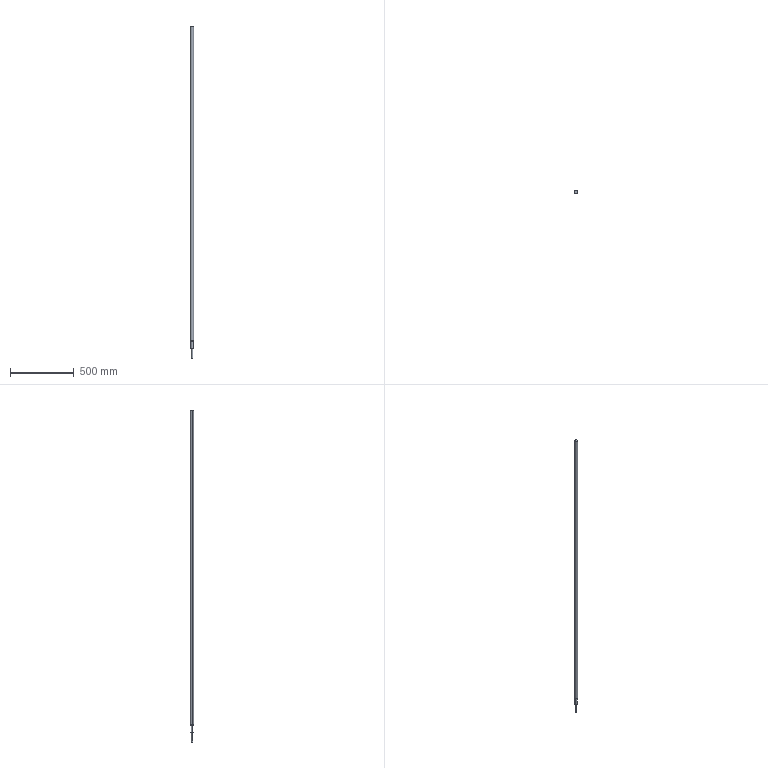Part | STEP file | _1-LCV02-25-5-L1400-F27-P101 | 1 solid | 14 faces | box 25 x 25 x 2604 mm | volume 1237665 mm3 | cylinder 6 | cone 4 | plane 4 | commonest cylinder face diameters 10 x2 20 x2 25 x2
STEP:
#1=CARTESIAN_POINT('',(12.5,0.,-1311.08));
#2=VERTEX_POINT('',#1);
#3=CARTESIAN_POINT('',(-12.5,0.,-1311.08));
#4=VERTEX_POINT('',#3);
#5=CARTESIAN_POINT('',(0.,0.,-1311.08));
#6=DIRECTION('',(0.,0.,1.));
#7=DIRECTION('',(1.,0.,0.));
#8=AXIS2_PLACEMENT_3D('',#5,#6,#7);
#9=CIRCLE('',#8,12.5);
#10=EDGE_CURVE('',#2,#4,#9,.T.);
#11=ORIENTED_EDGE('',*,*,#10,.T.);
#12=CARTESIAN_POINT('',(-12.5,0.,1159.));
#13=VERTEX_POINT('',#12);
#14=CARTESIAN_POINT('',(-12.5,0.,-1400.));
#15=DIRECTION('',(0.,0.,1.));
#16=VECTOR('',#15,1000.);
#17=LINE('',#14,#16);
#18=EDGE_CURVE('',#4,#13,#17,.T.);
#19=ORIENTED_EDGE('',*,*,#18,.T.);
#20=CARTESIAN_POINT('',(12.5,0.,1159.));
#21=VERTEX_POINT('',#20);
#22=CARTESIAN_POINT('',(0.,0.,1159.));
#23=DIRECTION('',(0.,0.,1.));
#24=DIRECTION('',(1.,0.,0.));
#25=AXIS2_PLACEMENT_3D('',#22,#23,#24);
#26=CIRCLE('',#25,12.5);
#27=EDGE_CURVE('',#21,#13,#26,.T.);
#28=ORIENTED_EDGE('',*,*,#27,.F.);
#29=CARTESIAN_POINT('',(12.5,0.,-1400.));
#30=DIRECTION('',(0.,0.,1.));
#31=VECTOR('',#30,1000.);
#32=LINE('',#29,#31);
#33=EDGE_CURVE('',#2,#21,#32,.T.);
#34=ORIENTED_EDGE('',*,*,#33,.F.);
#35=EDGE_LOOP('',(#11,#19,#28,#34));
#36=FACE_OUTER_BOUND('',#35,.T.);
#37=CARTESIAN_POINT('',(0.,0.,-1400.));
#38=DIRECTION('',(0.,0.,1.));
#39=DIRECTION('',(1.,0.,0.));
#40=AXIS2_PLACEMENT_3D('',#37,#38,#39);
#41=CYLINDRICAL_SURFACE('',#40,12.5);
#42=ADVANCED_FACE('',(#36),#41,.T.);
#43=CARTESIAN_POINT('',(11.58,0.,-1312.));
#44=VERTEX_POINT('',#43);
#45=CARTESIAN_POINT('',(-11.58,0.,-1312.));
#46=VERTEX_POINT('',#45);
#47=CARTESIAN_POINT('',(0.,0.,-1312.));
#48=DIRECTION('',(0.,0.,1.));
#49=DIRECTION('',(1.,0.,0.));
#50=AXIS2_PLACEMENT_3D('',#47,#48,#49);
#51=CIRCLE('',#50,11.58);
#52=EDGE_CURVE('',#44,#46,#51,.T.);
#53=ORIENTED_EDGE('',*,*,#52,.T.);
#54=CARTESIAN_POINT('',(-12.5,0.,-1311.08));
#55=DIRECTION('',(-0.7071,0.,0.7071));
#56=VECTOR('',#55,1000.);
#57=LINE('',#54,#56);
#58=EDGE_CURVE('',#46,#4,#57,.T.);
#59=ORIENTED_EDGE('',*,*,#58,.T.);
#60=ORIENTED_EDGE('',*,*,#10,.F.);
#61=CARTESIAN_POINT('',(12.5,0.,-1311.08));
#62=DIRECTION('',(0.7071,0.,0.7071));
#63=VECTOR('',#62,1000.);
#64=LINE('',#61,#63);
#65=EDGE_CURVE('',#44,#2,#64,.T.);
#66=ORIENTED_EDGE('',*,*,#65,.F.);
#67=EDGE_LOOP('',(#53,#59,#60,#66));
#68=FACE_OUTER_BOUND('',#67,.T.);
#69=CARTESIAN_POINT('',(0.,0.,-1311.08));
#70=DIRECTION('',(0.,0.,1.));
#71=DIRECTION('',(1.,0.,0.));
#72=AXIS2_PLACEMENT_3D('',#69,#70,#71);
#73=CONICAL_SURFACE('',#72,12.5,0.7854);
#74=ADVANCED_FACE('',(#68),#73,.T.);
#75=CARTESIAN_POINT('',(10.,0.,-1371.466));
#76=VERTEX_POINT('',#75);
#77=CARTESIAN_POINT('',(-10.,0.,-1371.466));
#78=VERTEX_POINT('',#77);
#79=CARTESIAN_POINT('',(0.,0.,-1371.466));
#80=DIRECTION('',(0.,0.,1.));
#81=DIRECTION('',(1.,0.,0.));
#82=AXIS2_PLACEMENT_3D('',#79,#80,#81);
#83=CIRCLE('',#82,10.);
#84=EDGE_CURVE('',#76,#78,#83,.T.);
#85=ORIENTED_EDGE('',*,*,#84,.T.);
#86=CARTESIAN_POINT('',(-10.,0.,-1312.));
#87=VERTEX_POINT('',#86);
#88=CARTESIAN_POINT('',(-10.,0.,-1400.));
#89=DIRECTION('',(0.,0.,1.));
#90=VECTOR('',#89,1000.);
#91=LINE('',#88,#90);
#92=EDGE_CURVE('',#78,#87,#91,.T.);
#93=ORIENTED_EDGE('',*,*,#92,.T.);
#94=CARTESIAN_POINT('',(10.,0.,-1312.));
#95=VERTEX_POINT('',#94);
#96=CARTESIAN_POINT('',(0.,0.,-1312.));
#97=DIRECTION('',(0.,0.,-1.));
#98=DIRECTION('',(1.,0.,0.));
#99=AXIS2_PLACEMENT_3D('',#96,#97,#98);
#100=CIRCLE('',#99,10.);
#101=EDGE_CURVE('',#87,#95,#100,.T.);
#102=ORIENTED_EDGE('',*,*,#101,.T.);
#103=CARTESIAN_POINT('',(10.,0.,-1400.));
#104=DIRECTION('',(0.,0.,1.));
#105=VECTOR('',#104,1000.);
#106=LINE('',#103,#105);
#107=EDGE_CURVE('',#76,#95,#106,.T.);
#108=ORIENTED_EDGE('',*,*,#107,.F.);
#109=EDGE_LOOP('',(#85,#93,#102,#108));
#110=FACE_OUTER_BOUND('',#109,.T.);
#111=CARTESIAN_POINT('',(0.,0.,-1400.));
#112=DIRECTION('',(0.,0.,1.));
#113=DIRECTION('',(1.,0.,0.));
#114=AXIS2_PLACEMENT_3D('',#111,#112,#113);
#115=CYLINDRICAL_SURFACE('',#114,10.);
#116=ADVANCED_FACE('',(#110),#115,.T.);
#117=CARTESIAN_POINT('',(8.466,0.,-1373.));
#118=VERTEX_POINT('',#117);
#119=CARTESIAN_POINT('',(-8.466,0.,-1373.));
#120=VERTEX_POINT('',#119);
#121=CARTESIAN_POINT('',(0.,0.,-1373.));
#122=DIRECTION('',(0.,0.,1.));
#123=DIRECTION('',(1.,0.,0.));
#124=AXIS2_PLACEMENT_3D('',#121,#122,#123);
#125=CIRCLE('',#124,8.466);
#126=EDGE_CURVE('',#118,#120,#125,.T.);
#127=ORIENTED_EDGE('',*,*,#126,.T.);
#128=CARTESIAN_POINT('',(-10.,0.,-1371.466));
#129=DIRECTION('',(-0.7071,0.,0.7071));
#130=VECTOR('',#129,1000.);
#131=LINE('',#128,#130);
#132=EDGE_CURVE('',#120,#78,#131,.T.);
#133=ORIENTED_EDGE('',*,*,#132,.T.);
#134=ORIENTED_EDGE('',*,*,#84,.F.);
#135=CARTESIAN_POINT('',(10.,0.,-1371.466));
#136=DIRECTION('',(0.7071,0.,0.7071));
#137=VECTOR('',#136,1000.);
#138=LINE('',#135,#137);
#139=EDGE_CURVE('',#118,#76,#138,.T.);
#140=ORIENTED_EDGE('',*,*,#139,.F.);
#141=EDGE_LOOP('',(#127,#133,#134,#140));
#142=FACE_OUTER_BOUND('',#141,.T.);
#143=CARTESIAN_POINT('',(0.,0.,-1371.466));
#144=DIRECTION('',(0.,0.,1.));
#145=DIRECTION('',(1.,0.,0.));
#146=AXIS2_PLACEMENT_3D('',#143,#144,#145);
#147=CONICAL_SURFACE('',#146,10.,0.7854);
#148=ADVANCED_FACE('',(#142),#147,.T.);
#149=CARTESIAN_POINT('',(-5.,0.,-1445.));
#150=VERTEX_POINT('',#149);
#151=CARTESIAN_POINT('',(5.,0.,-1445.));
#152=VERTEX_POINT('',#151);
#153=CARTESIAN_POINT('',(0.,0.,-1445.));
#154=DIRECTION('',(0.,0.,-1.));
#155=DIRECTION('',(-1.,0.,0.));
#156=AXIS2_PLACEMENT_3D('',#153,#154,#155);
#157=CIRCLE('',#156,5.);
#158=EDGE_CURVE('',#150,#152,#157,.T.);
#159=ORIENTED_EDGE('',*,*,#158,.F.);
#160=CARTESIAN_POINT('',(-5.,0.,-1373.));
#161=VERTEX_POINT('',#160);
#162=CARTESIAN_POINT('',(-5.,0.,-1400.));
#163=DIRECTION('',(0.,0.,1.));
#164=VECTOR('',#163,1000.);
#165=LINE('',#162,#164);
#166=EDGE_CURVE('',#150,#161,#165,.T.);
#167=ORIENTED_EDGE('',*,*,#166,.T.);
#168=CARTESIAN_POINT('',(5.,0.,-1373.));
#169=VERTEX_POINT('',#168);
#170=CARTESIAN_POINT('',(0.,0.,-1373.));
#171=DIRECTION('',(0.,0.,-1.));
#172=DIRECTION('',(1.,0.,0.));
#173=AXIS2_PLACEMENT_3D('',#170,#171,#172);
#174=CIRCLE('',#173,5.);
#175=EDGE_CURVE('',#161,#169,#174,.T.);
#176=ORIENTED_EDGE('',*,*,#175,.T.);
#177=CARTESIAN_POINT('',(5.,0.,-1400.));
#178=DIRECTION('',(0.,0.,1.));
#179=VECTOR('',#178,1000.);
#180=LINE('',#177,#179);
#181=EDGE_CURVE('',#152,#169,#180,.T.);
#182=ORIENTED_EDGE('',*,*,#181,.F.);
#183=EDGE_LOOP('',(#159,#167,#176,#182));
#184=FACE_OUTER_BOUND('',#183,.T.);
#185=CARTESIAN_POINT('',(0.,0.,-1400.));
#186=DIRECTION('',(0.,0.,1.));
#187=DIRECTION('',(1.,0.,0.));
#188=AXIS2_PLACEMENT_3D('',#185,#186,#187);
#189=CYLINDRICAL_SURFACE('',#188,5.);
#190=ADVANCED_FACE('',(#184),#189,.T.);
#191=ORIENTED_EDGE('',*,*,#27,.T.);
#192=CARTESIAN_POINT('',(0.,0.,1159.));
#193=DIRECTION('',(0.,0.,1.));
#194=DIRECTION('',(1.,0.,0.));
#195=AXIS2_PLACEMENT_3D('',#192,#193,#194);
#196=CIRCLE('',#195,12.5);
#197=EDGE_CURVE('',#13,#21,#196,.T.);
#198=ORIENTED_EDGE('',*,*,#197,.T.);
#199=EDGE_LOOP('',(#191,#198));
#200=FACE_OUTER_BOUND('',#199,.T.);
#201=CARTESIAN_POINT('',(0.,0.,1159.));
#202=DIRECTION('',(0.,0.,1.));
#203=DIRECTION('',(1.,0.,0.));
#204=AXIS2_PLACEMENT_3D('',#201,#202,#203);
#205=PLANE('',#204);
#206=ADVANCED_FACE('',(#200),#205,.T.);
#207=ORIENTED_EDGE('',*,*,#18,.F.);
#208=CARTESIAN_POINT('',(0.,0.,-1311.08));
#209=DIRECTION('',(0.,0.,1.));
#210=DIRECTION('',(1.,0.,0.));
#211=AXIS2_PLACEMENT_3D('',#208,#209,#210);
#212=CIRCLE('',#211,12.5);
#213=EDGE_CURVE('',#4,#2,#212,.T.);
#214=ORIENTED_EDGE('',*,*,#213,.T.);
#215=ORIENTED_EDGE('',*,*,#33,.T.);
#216=ORIENTED_EDGE('',*,*,#197,.F.);
#217=EDGE_LOOP('',(#207,#214,#215,#216));
#218=FACE_OUTER_BOUND('',#217,.T.);
#219=CARTESIAN_POINT('',(0.,0.,-1400.));
#220=DIRECTION('',(0.,0.,1.));
#221=DIRECTION('',(1.,0.,0.));
#222=AXIS2_PLACEMENT_3D('',#219,#220,#221);
#223=CYLINDRICAL_SURFACE('',#222,12.5);
#224=ADVANCED_FACE('',(#218),#223,.T.);
#225=ORIENTED_EDGE('',*,*,#58,.F.);
#226=CARTESIAN_POINT('',(0.,0.,-1312.));
#227=DIRECTION('',(0.,0.,1.));
#228=DIRECTION('',(1.,0.,0.));
#229=AXIS2_PLACEMENT_3D('',#226,#227,#228);
#230=CIRCLE('',#229,11.58);
#231=EDGE_CURVE('',#46,#44,#230,.T.);
#232=ORIENTED_EDGE('',*,*,#231,.T.);
#233=ORIENTED_EDGE('',*,*,#65,.T.);
#234=ORIENTED_EDGE('',*,*,#213,.F.);
#235=EDGE_LOOP('',(#225,#232,#233,#234));
#236=FACE_OUTER_BOUND('',#235,.T.);
#237=CARTESIAN_POINT('',(0.,0.,-1311.08));
#238=DIRECTION('',(0.,0.,1.));
#239=DIRECTION('',(1.,0.,0.));
#240=AXIS2_PLACEMENT_3D('',#237,#238,#239);
#241=CONICAL_SURFACE('',#240,12.5,0.7854);
#242=ADVANCED_FACE('',(#236),#241,.T.);
#243=ORIENTED_EDGE('',*,*,#52,.F.);
#244=ORIENTED_EDGE('',*,*,#231,.F.);
#245=EDGE_LOOP('',(#243,#244));
#246=FACE_OUTER_BOUND('',#245,.T.);
#247=CARTESIAN_POINT('',(0.,0.,-1312.));
#248=DIRECTION('',(0.,0.,-1.));
#249=DIRECTION('',(1.,0.,0.));
#250=AXIS2_PLACEMENT_3D('',#247,#248,#249);
#251=CIRCLE('',#250,10.);
#252=EDGE_CURVE('',#95,#87,#251,.T.);
#253=ORIENTED_EDGE('',*,*,#252,.F.);
#254=ORIENTED_EDGE('',*,*,#101,.F.);
#255=EDGE_LOOP('',(#253,#254));
#256=FACE_BOUND('',#255,.T.);
#257=CARTESIAN_POINT('',(0.,11.58,-1312.));
#258=DIRECTION('',(0.,0.,1.));
#259=DIRECTION('',(1.,0.,0.));
#260=AXIS2_PLACEMENT_3D('',#257,#258,#259);
#261=PLANE('',#260);
#262=ADVANCED_FACE('',(#246,#256),#261,.F.);
#263=ORIENTED_EDGE('',*,*,#92,.F.);
#264=CARTESIAN_POINT('',(0.,0.,-1371.466));
#265=DIRECTION('',(0.,0.,1.));
#266=DIRECTION('',(1.,0.,0.));
#267=AXIS2_PLACEMENT_3D('',#264,#265,#266);
#268=CIRCLE('',#267,10.);
#269=EDGE_CURVE('',#78,#76,#268,.T.);
#270=ORIENTED_EDGE('',*,*,#269,.T.);
#271=ORIENTED_EDGE('',*,*,#107,.T.);
#272=ORIENTED_EDGE('',*,*,#252,.T.);
#273=EDGE_LOOP('',(#263,#270,#271,#272));
#274=FACE_OUTER_BOUND('',#273,.T.);
#275=CARTESIAN_POINT('',(0.,0.,-1400.));
#276=DIRECTION('',(0.,0.,1.));
#277=DIRECTION('',(1.,0.,0.));
#278=AXIS2_PLACEMENT_3D('',#275,#276,#277);
#279=CYLINDRICAL_SURFACE('',#278,10.);
#280=ADVANCED_FACE('',(#274),#279,.T.);
#281=ORIENTED_EDGE('',*,*,#132,.F.);
#282=CARTESIAN_POINT('',(0.,0.,-1373.));
#283=DIRECTION('',(0.,0.,1.));
#284=DIRECTION('',(1.,0.,0.));
#285=AXIS2_PLACEMENT_3D('',#282,#283,#284);
#286=CIRCLE('',#285,8.466);
#287=EDGE_CURVE('',#120,#118,#286,.T.);
#288=ORIENTED_EDGE('',*,*,#287,.T.);
#289=ORIENTED_EDGE('',*,*,#139,.T.);
#290=ORIENTED_EDGE('',*,*,#269,.F.);
#291=EDGE_LOOP('',(#281,#288,#289,#290));
#292=FACE_OUTER_BOUND('',#291,.T.);
#293=CARTESIAN_POINT('',(0.,0.,-1371.466));
#294=DIRECTION('',(0.,0.,1.));
#295=DIRECTION('',(1.,0.,0.));
#296=AXIS2_PLACEMENT_3D('',#293,#294,#295);
#297=CONICAL_SURFACE('',#296,10.,0.7854);
#298=ADVANCED_FACE('',(#292),#297,.T.);
#299=ORIENTED_EDGE('',*,*,#126,.F.);
#300=ORIENTED_EDGE('',*,*,#287,.F.);
#301=EDGE_LOOP('',(#299,#300));
#302=FACE_OUTER_BOUND('',#301,.T.);
#303=CARTESIAN_POINT('',(0.,0.,-1373.));
#304=DIRECTION('',(0.,0.,-1.));
#305=DIRECTION('',(1.,0.,0.));
#306=AXIS2_PLACEMENT_3D('',#303,#304,#305);
#307=CIRCLE('',#306,5.);
#308=EDGE_CURVE('',#169,#161,#307,.T.);
#309=ORIENTED_EDGE('',*,*,#308,.F.);
#310=ORIENTED_EDGE('',*,*,#175,.F.);
#311=EDGE_LOOP('',(#309,#310));
#312=FACE_BOUND('',#311,.T.);
#313=CARTESIAN_POINT('',(0.,8.466,-1373.));
#314=DIRECTION('',(0.,0.,1.));
#315=DIRECTION('',(1.,0.,0.));
#316=AXIS2_PLACEMENT_3D('',#313,#314,#315);
#317=PLANE('',#316);
#318=ADVANCED_FACE('',(#302,#312),#317,.F.);
#319=ORIENTED_EDGE('',*,*,#166,.F.);
#320=CARTESIAN_POINT('',(0.,0.,-1445.));
#321=DIRECTION('',(0.,0.,-1.));
#322=DIRECTION('',(-1.,0.,0.));
#323=AXIS2_PLACEMENT_3D('',#320,#321,#322);
#324=CIRCLE('',#323,5.);
#325=EDGE_CURVE('',#152,#150,#324,.T.);
#326=ORIENTED_EDGE('',*,*,#325,.F.);
#327=ORIENTED_EDGE('',*,*,#181,.T.);
#328=ORIENTED_EDGE('',*,*,#308,.T.);
#329=EDGE_LOOP('',(#319,#326,#327,#328));
#330=FACE_OUTER_BOUND('',#329,.T.);
#331=CARTESIAN_POINT('',(0.,0.,-1400.));
#332=DIRECTION('',(0.,0.,1.));
#333=DIRECTION('',(1.,0.,0.));
#334=AXIS2_PLACEMENT_3D('',#331,#332,#333);
#335=CYLINDRICAL_SURFACE('',#334,5.);
#336=ADVANCED_FACE('',(#330),#335,.T.);
#337=ORIENTED_EDGE('',*,*,#325,.T.);
#338=ORIENTED_EDGE('',*,*,#158,.T.);
#339=EDGE_LOOP('',(#337,#338));
#340=FACE_OUTER_BOUND('',#339,.T.);
#341=CARTESIAN_POINT('',(0.,0.,-1445.));
#342=DIRECTION('',(0.,0.,-1.));
#343=DIRECTION('',(-1.,0.,0.));
#344=AXIS2_PLACEMENT_3D('',#341,#342,#343);
#345=PLANE('',#344);
#346=ADVANCED_FACE('',(#340),#345,.T.);
#347=CLOSED_SHELL('',(#42,#74,#116,#148,#190,#206,#224,#242,#262,#280,#298,#318,#336,#346));
#348=MANIFOLD_SOLID_BREP('',#347);
#349=CARTESIAN_POINT('',(0.,0.,0.));
#350=DIRECTION('',(0.,0.,1.));
#351=DIRECTION('',(1.,0.,0.));
#352=AXIS2_PLACEMENT_3D('',#349,#350,#351);
#353=(LENGTH_UNIT()NAMED_UNIT(*)SI_UNIT(.MILLI.,.METRE.));
#354=UNCERTAINTY_MEASURE_WITH_UNIT(LENGTH_MEASURE(0.00001),#353,'','');
#355=(NAMED_UNIT(*)PLANE_ANGLE_UNIT()SI_UNIT($,.RADIAN.));
#356=(NAMED_UNIT(*)SI_UNIT($,.STERADIAN.)SOLID_ANGLE_UNIT());
#357=(GEOMETRIC_REPRESENTATION_CONTEXT(3)GLOBAL_UNCERTAINTY_ASSIGNED_CONTEXT((#354))GLOBAL_UNIT_ASSIGNED_CONTEXT((#353,#355,#356))REPRESENTATION_CONTEXT('',''));
#358=ADVANCED_BREP_SHAPE_REPRESENTATION('',(#348,#352),#357);